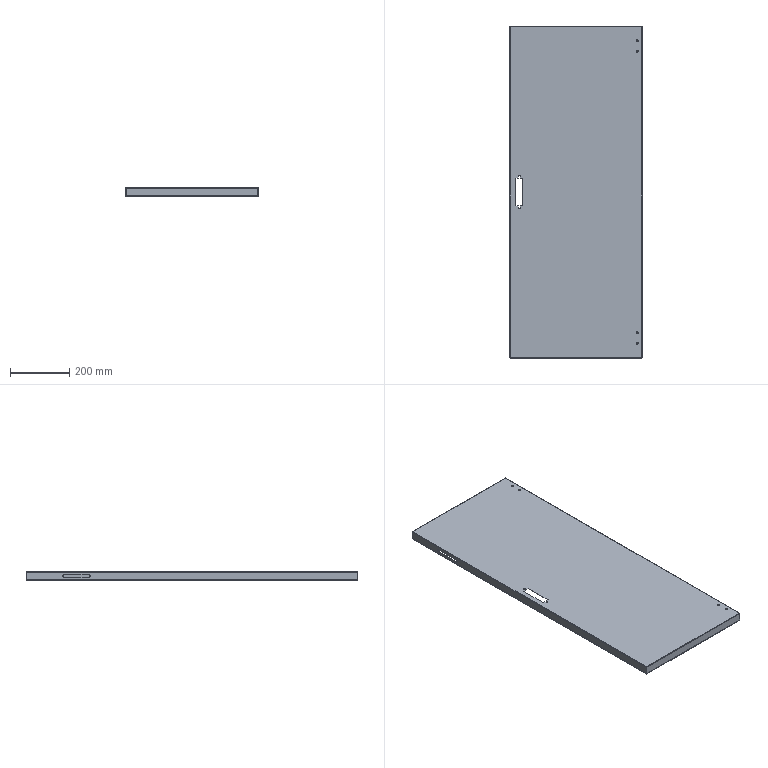Part | 1 solid | 95 faces | box 447 x 1120 x 30 mm | volume 740612 mm3 | plane 50 | cylinder 29 | spline 16 | commonest cylinder face diameters 7 x13 1.473 x8 3.873 x8